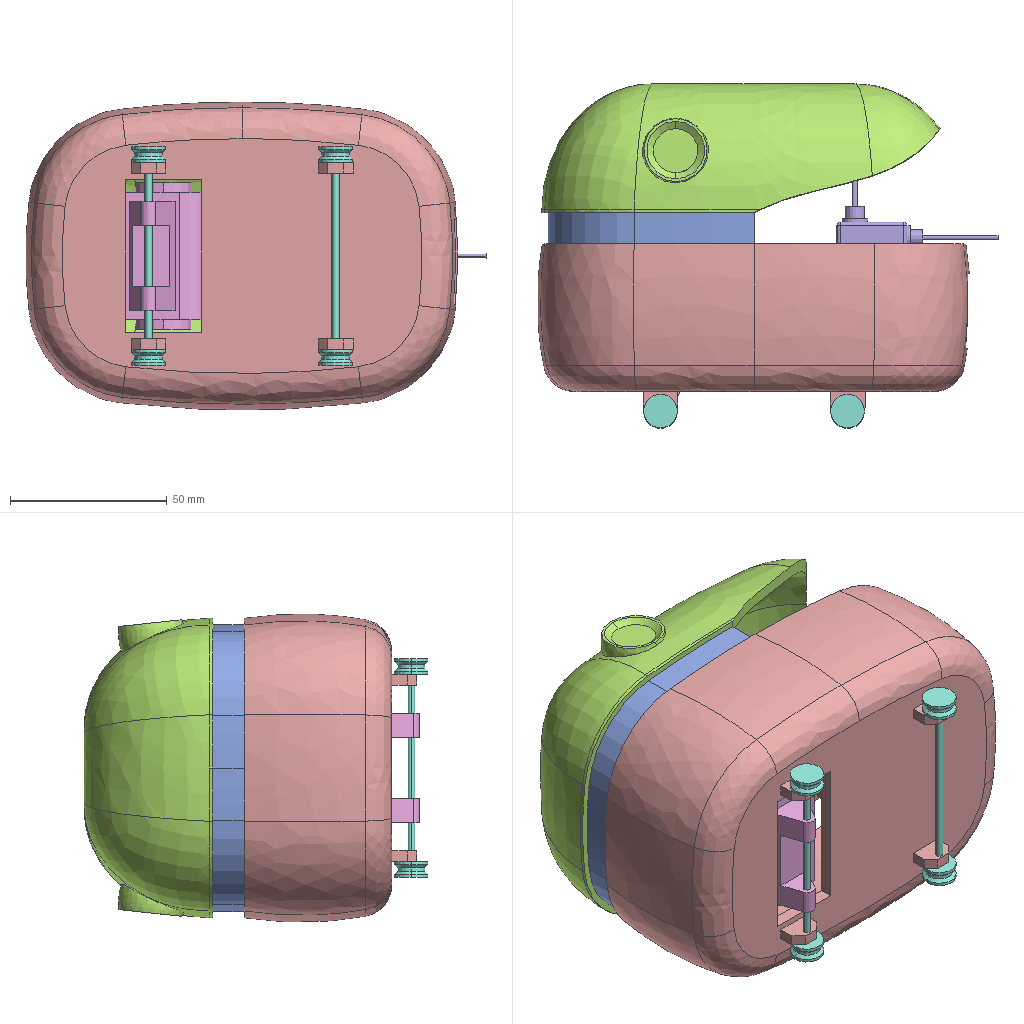Assembly | SolidWorks | 5 different items | 6 placed | box 147 x 110 x 98 mm
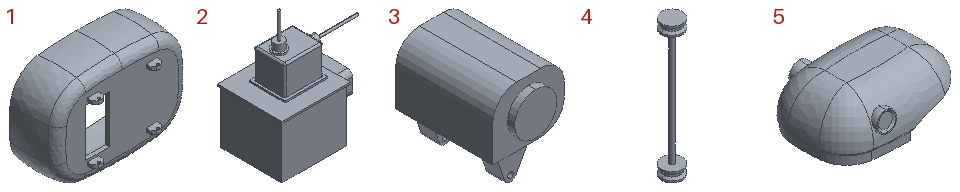Parts list (item | quantity | size | volume | features):
1 | x1 | 137.558 x 55 x 98.119 mm | 101506 mm3 | features Cut 4, MirrorPattern 2, Chamfer 1, Extrusion 1, Fillet 1, ICE 1, Shell 1, Sweep 1
2 | x1 | 62.713 x 37.625 x 70 mm | 50756 mm3 | features ICE 10, Extrusion 1, Fillet 1
3 | x1 | 29.956 x 46.658 x 37.777 mm | 31870 mm3 | features ICE 3, Cut 1, Extrusion 1, Fillet 1
4 | x2 | 10.836 x 10.836 x 69.732 mm | 1053 mm3 | features Extrusion 1, ICE 1, MirrorPattern 1, RefAxis 1, RevCut 1
5 | x1 | 126.879 x 95.425 x 51 mm | 71038 mm3 | features DelFace 2, Cut 1, Extrusion 1, Fillet 1, ICE 1, MirrorPattern 1, Revolution 1, Shell 1
Mates (type | each side: item.copy, entity, surface, feature):
InPlace | 1.1 face plane Boss-Extrude2 | 5.1 plane
InPlace | 1.1 face plane Shell3 | 3.1 plane
InPlace | 1.1 face plane Boss-Extrude3 | 4.1 plane
Concentric | 1.1 face cylinder Mirror3 | 4.2 face cylinder Boss-Extrude1
Coincident | 1.1 face plane Mirror3 | 4.2 face plane Mirror1
InPlace | 1.1 face plane Shell3 | 2.1 plane